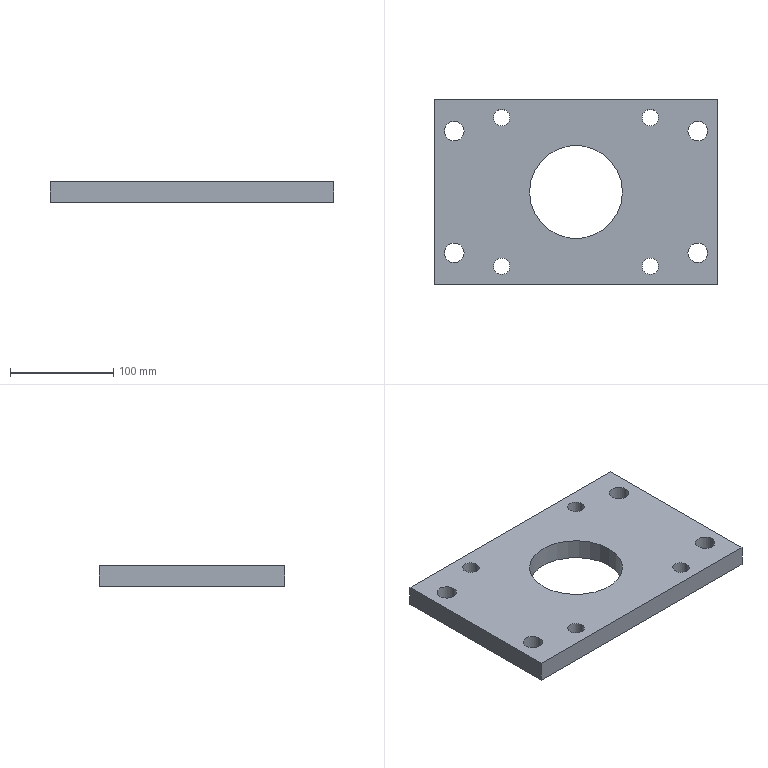Part | STEP file | CDS1FN160-250-A54Z_CS1-Flange | 1 solid | 24 faces | box 275 x 180 x 20 mm | volume 823998 mm3 | cylinder 18 | plane 6 | commonest cylinder face diameters 16 x8 19 x8 90 x2